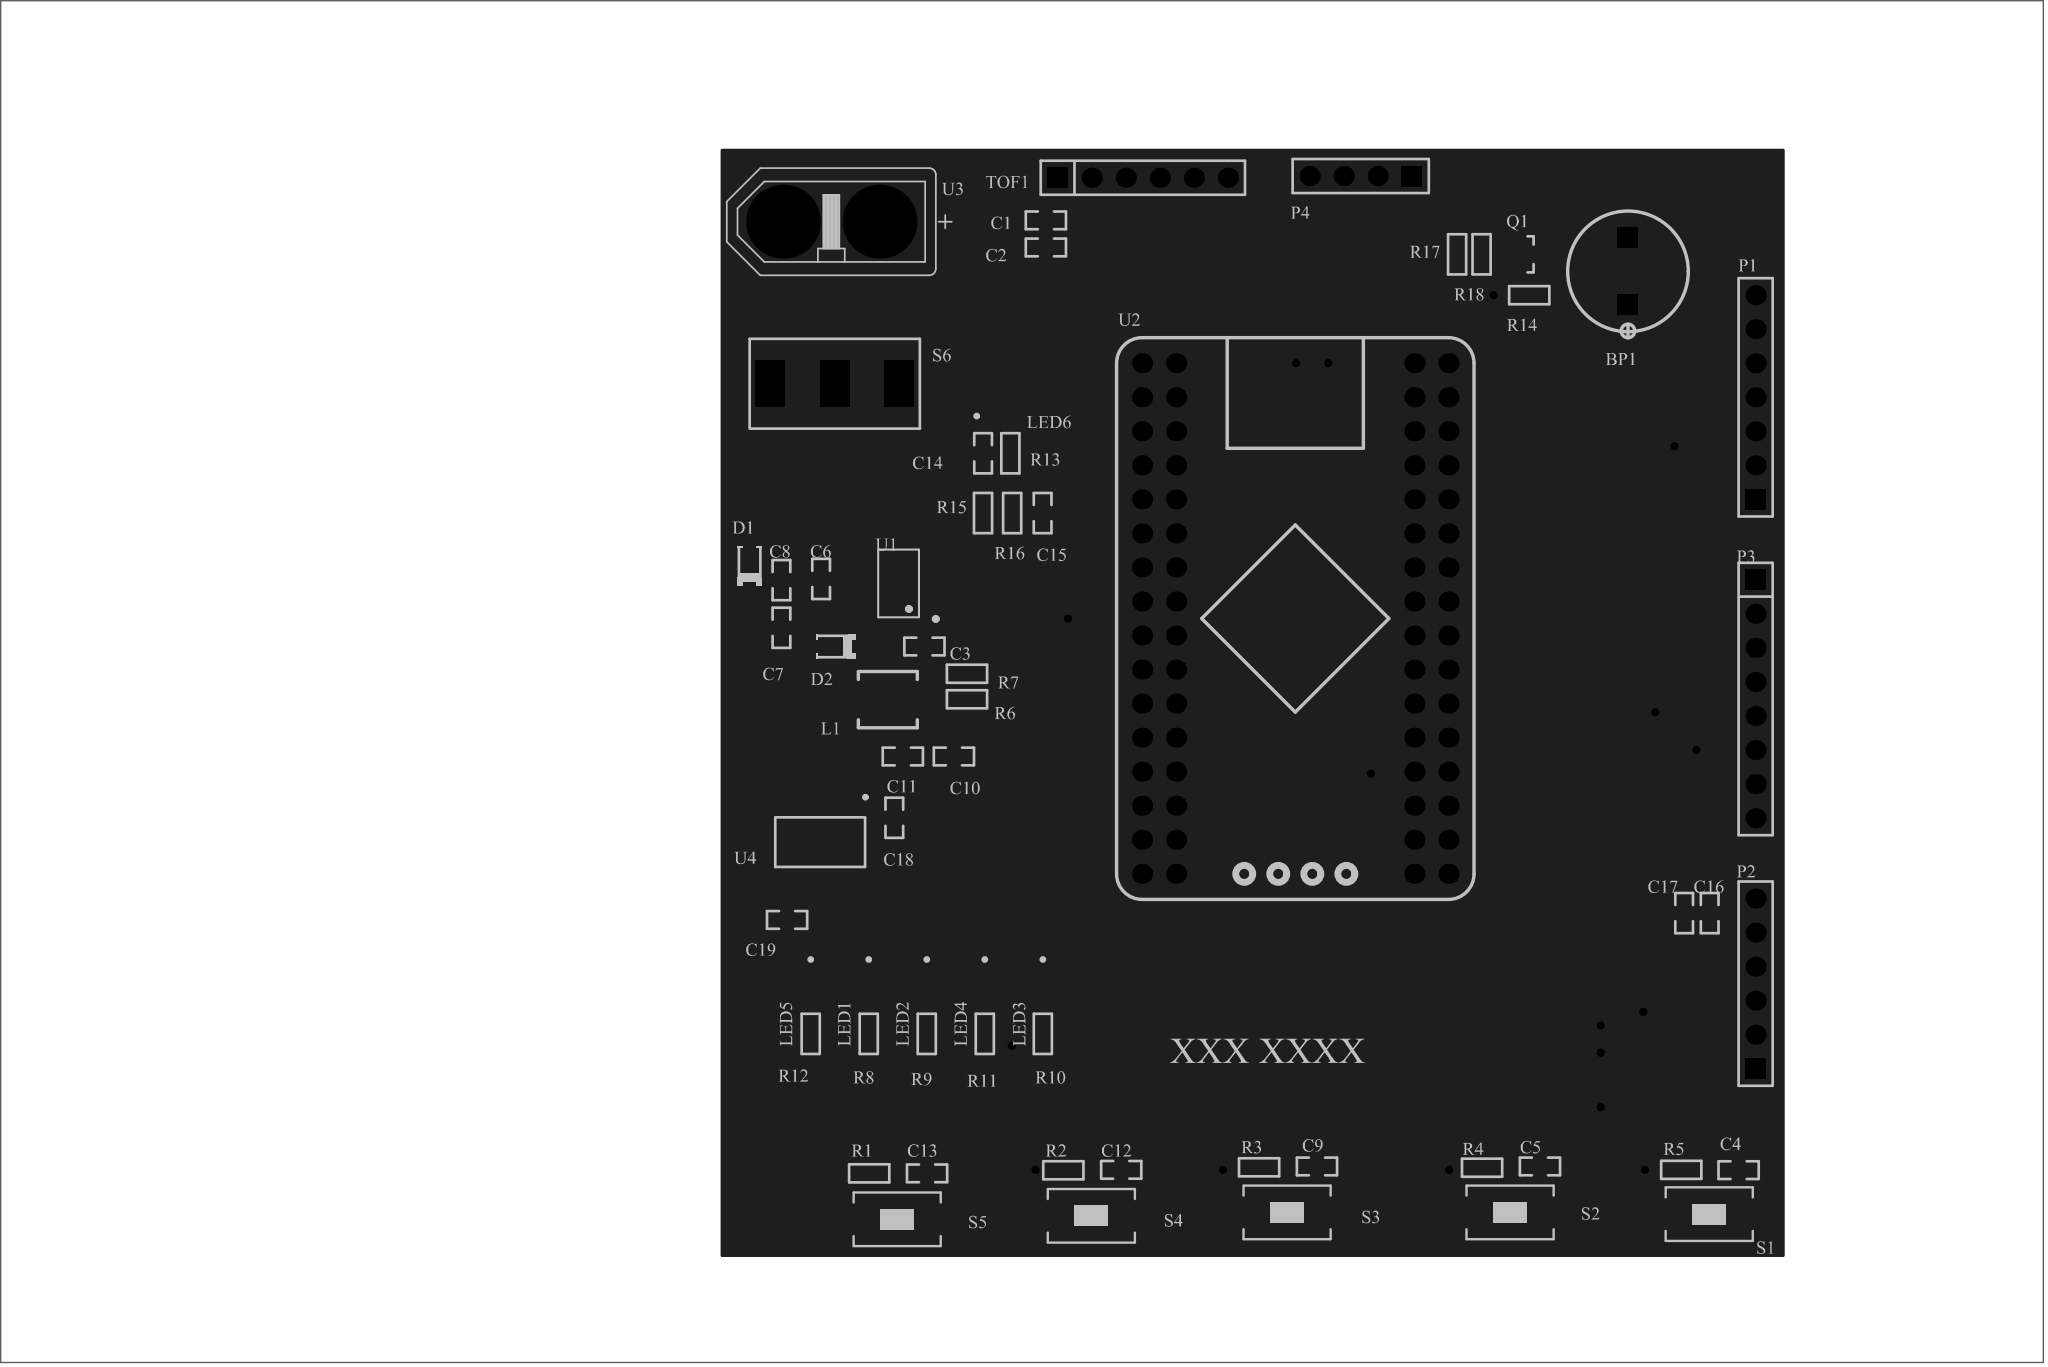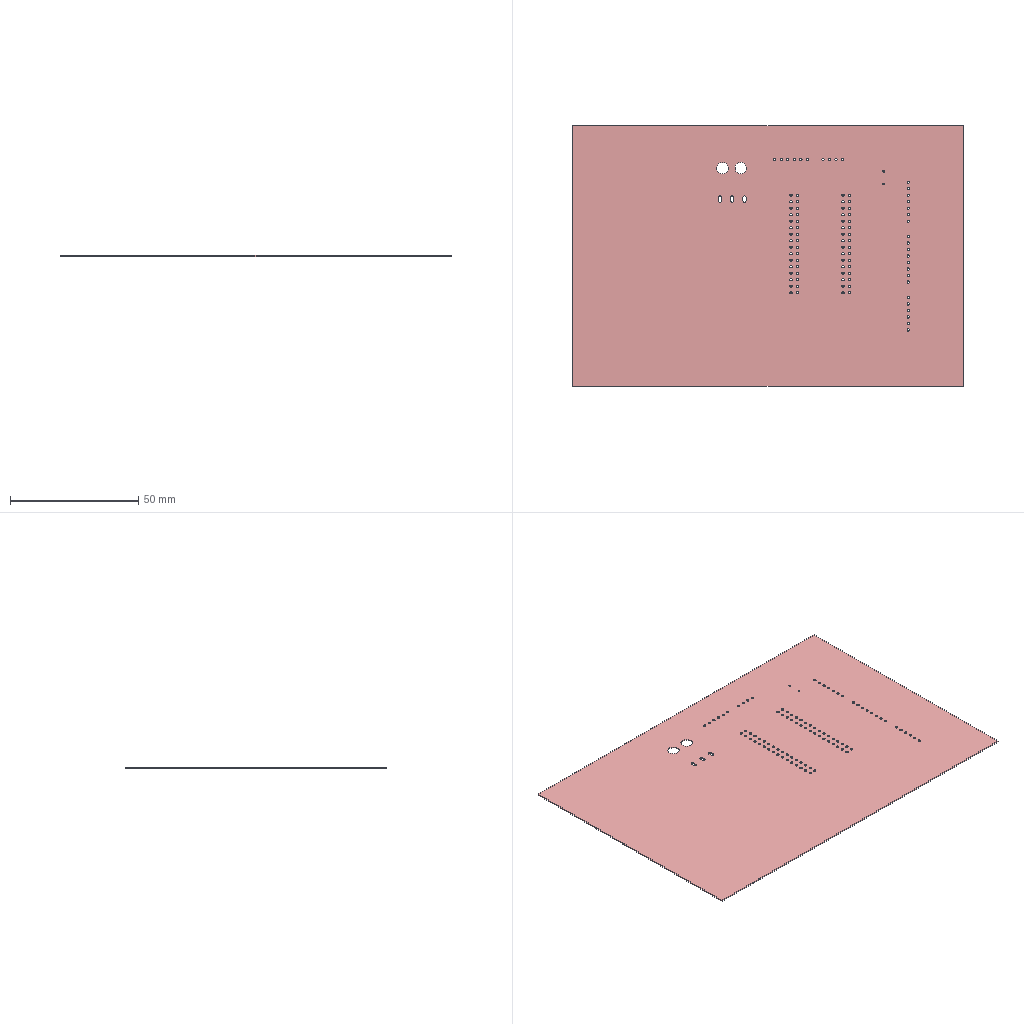Circuit board layout | Altium Designer | box 152.4 x 101.6 x 0.4 mm
Layer stack:
# Altium Designer layer stack of  (unit mm; dielectric type: 0 none, 1 core, 2 prepreg, 3 surface material)
index,name,kind,layer,copper_thickness_mm,dielectric_type,dielectric_thickness_mm,dielectric_material,dielectric_constant
0,Top Paste Mask Layer,other,,,,,,
1,Top Silkscreen Layer,other,,,,,,
2,Top Solder Mask Layer,dielectric,,,3,0.0102,Solder Resist,3.5
3,Top Layer,copper,Top Layer,0.0356,,,,
4,Dielectric 1,dielectric,,,3,0.32,FR-4,4.8
5,Bottom Layer,copper,Bottom Layer,0.0356,,,,
6,Bottom Solder Mask Layer,dielectric,,,3,0.0102,Solder Resist,3.5
7,Bottom Silkscreen Layer,other,,,,,,
8,Bottom Paste Mask Layer,other,,,,,,
# drill layer pairs: low layer,high layer
drill_pair,Top Layer,Bottom Layer
Part placement:
Designator,Comment,Layer,Footprint,Center-X(mm),Center-Y(mm),Rotation
U4,LM1117,TopLayer,LM1117_-_duplicate,137.342,115.023,180
U3,XT60-F,TopLayer,XT60,138.174,161.311,0
U2,STC32G12K128,TopLayer,STC16F40K128_CoreBoard,172.791,131.705,0
U1,TPS5450,TopLayer,5450,143.193,134.324,90
TOF1,Ranging module,TopLayer,HDR1X6,161.417,164.592,0
S6,SW,TopLayer,SS12D10,138.43,149.225,0
S5,KEY,TopLayer,anjiantiepiankaiguan,143.087,86.882,0
S4,KEY,TopLayer,anjiantiepiankaiguan,157.573,87.144,0
S3,KEY,TopLayer,anjiantiepiankaiguan,172.178,87.398,0
S2,KEY,TopLayer,anjiantiepiankaiguan,188.815,87.398,0
S1,KEY,TopLayer,anjiantiepiankaiguan,203.674,87.271,0
R18,10K ±1%,TopLayer,RESC1608[0603]S-N,186.69,158.877,270
R17,4.7K ±1%,TopLayer,RESC1608[0603]S-N,184.863,158.878,90
R16,1K ±1%,TopLayer,RESC1608[0603]S-N,151.667,139.573,90
R15,10K ±1%,TopLayer,RESC1608[0603]S-N,149.494,139.573,270
R14,10R ±1%,TopLayer,RESC1608[0603]S-N,190.246,155.829,0
R13,1K,TopLayer,RESC1608[0603]S-N,151.533,144.036,90
R12,10K,TopLayer,RESC1608[0603]S-N,136.636,100.718,90
R11,10K,TopLayer,RESC1608[0603]S-N,149.626,100.718,90
R10,10K,TopLayer,RESC1608[0603]S-N,153.956,100.718,90
R9,10K,TopLayer,RESC1608[0603]S-N,145.296,100.718,90
R8,10K,TopLayer,RESC1608[0603]S-N,140.966,100.718,90
R7,3K,TopLayer,RESC1608[0603]S-N,148.296,127.586,180
R6,10K,TopLayer,RESC1608[0603]S-N,148.296,125.681,180
R5,1K,TopLayer,RESC1608[0603]S-N,201.586,90.573,180
R4,1K,TopLayer,RESC1608[0603]S-N,186.727,90.731,180
R3,1K,TopLayer,RESC1608[0603]S-N,170.09,90.763,180
R2,1K,TopLayer,RESC1608[0603]S-N,155.485,90.541,180
R1,1K,TopLayer,RESC1608[0603]S-N,140.999,90.311,180
Q1,S8050,TopLayer,SOT-23,189.987,158.878,0
P4,Header-D-M 1x4P,TopLayer,HDR1X4,177.673,164.719,180
P3,Header  1X8,TopLayer,HDR1X8,207.137,125.702,270
P2,Gyroscope,TopLayer,HDR1X6,207.137,104.465,90
P1,Header 7,TopLayer,HDR1X7,207.137,148.209,90
LED6,LED,TopLayer,LEDC1608(0603),150.622,146.812,0
LED5,LED,TopLayer,LEDC1608(0603),136.636,104.667,270
LED4,LED,TopLayer,LEDC1608(0603),149.626,104.667,270
LED3,LED,TopLayer,LEDC1608(0603),153.956,104.667,270
LED2,LED,TopLayer,LEDC1608(0603),145.296,104.667,270
LED1,LED,TopLayer,LEDC1608(0603),140.966,104.667,270
L1,4.7uH 2.5A,TopLayer,0402_TPC_4*4*2,142.389,125.655,270
D2,SS54,TopLayer,SOD-123-L,138.517,129.618,0
D1,SS54,TopLayer,SOD-123-L,132.08,135.636,270
C19,1uF,TopLayer,CAPC1608[0603]S-N,134.874,109.22,0
C18,1uF,TopLayer,CAPC1608[0603]S-N,142.875,116.84,270
C17,10uF ±10% 50V,TopLayer,CAPC1608[0603]S-N,201.803,109.728,270
C16,0.1uF ±10% 25V,TopLayer,CAPC1608[0603]S-N,203.708,109.728,270
C15,100nF 50V X7R,TopLayer,CAPC1608[0603]S-N,153.939,139.573,90
C14,1000uF  25V,TopLayer,CAPC1608[0603]S-N,149.498,144.036,90
C13,10uF,TopLayer,CAPC1608[0603]S-N,145.317,90.311,0
C12,10uF,TopLayer,CAPC1608[0603]S-N,159.803,90.573,0
C11,0.1uF,TopLayer,CAPC1608[0603]S-N,143.51,121.412,0
C10,100uF,TopLayer,CAPC1608[0603]S-N,147.32,121.412,0
C9,10uF,TopLayer,CAPC1608[0603]S-N,174.408,90.827,0
C8,4.7uF,TopLayer,CAPC1608[0603]S-N,134.453,134.571,270
C7,4.7uF,TopLayer,CAPC1608[0603]S-N,134.453,131.015,90
C6,0.1uF,TopLayer,CAPC1608[0603]S-N,137.413,134.659,270
C5,10uF,TopLayer,CAPC1608[0603]S-N,191.045,90.827,0
C4,10uF,TopLayer,CAPC1608[0603]S-N,205.867,90.551,0
C3,100nF,TopLayer,CAPC1608[0603]S-N,145.121,129.618,180
C2,0.1uF,TopLayer,CAPC1608[0603]S-N,154.182,159.391,0
C1,10uF,TopLayer,CAPC1608[0603]S-N,154.182,161.412,0
BP1,Buzzer,TopLayer,5*10fengmiqi,197.612,157.607,90
Pad and via stacks:
# Altium Designer via and pad stacks of  (unit mm). Each distinct definition once, with the count of objects using it.
# via: kind,start_layer,end_layer,hole_mm,diameter_mm,mode(0 simple;1 top-mid-bottom;2 full stack),diameter_per_layer,count,example_net
# pad: kind,layer,hole_mm,hole_type(0 round;1 square;2 slot),plating,top_size,top_shape(1 round;2 rect;3 octagon;9 rounded rect),mid_size,bottom_size,mode,footprint,size_per_layer,count,example
pad,Top Layer,0,0,plated,1.1x1.55,2,1.1x1.55,1.1x1.55,0,LM1117 - duplicate,,3,U4.2
pad,Top Layer,0,0,plated,3.45x1.55,2,3.45x1.55,3.45x1.55,0,LM1117 - duplicate,,1,U4.4
pad,Top Layer,0,0,plated,0.6x1.8,1,0.6x1.8,0.6x1.8,0,5450,,8,U1.1
pad,Top Layer,0,0,plated,2.29x2.29,2,2.29x2.29,2.29x2.29,0,5450,,1,U1.9
pad,Top Layer,0,0,plated,2.5x2,2,2.5x2,2.5x2,0,anjiantiepiankaiguan,,10,S5.2
pad,Top Layer,0,0,plated,0.95x0.9,2,0.95x0.9,0.95x0.9,0,RESC1608[0603]S-N,,36,R18.2
pad,Top Layer,0,0,plated,0.65x1.05,2,0.65x1.05,0.65x1.05,0,SOT-23,,3,Q1.3
pad,Top Layer,0,0,unplated,0.8x0.85,2,0.8x0.85,0.8x0.85,0,LEDC1608(0603),,12,LED6.A
pad,Top Layer,0,2,plated,1.5x2.5,2,1.5x2.5,1.5x2.5,0,0402 TPC 4*4*2,,2,L1.2
pad,Top Layer,0,0,unplated,1x0.85,2,1x0.85,1x0.85,0,SOD-123-L,,4,D2.K
pad,Top Layer,0,0,plated,0.95x0.9,2,0.95x0.9,0.95x0.9,0,CAPC1608[0603]S-N,,38,C19.1
pad,Multi-Layer,4.5,2,plated,5.516x5.516,1,5.516x5.516,5.516x5.516,0,XT60,,2,U3.
pad,Multi-Layer,0.9,0,plated,1.5x1.5,1,1.5x1.5,1.5x1.5,0,STC16F40K128_CoreBoard,,64,U2.40
pad,Multi-Layer,0.9,0,plated,1.5x1.5,1,1.5x1.5,1.5x1.5,0,HDR1X6,,10,TOF1.6
pad,Multi-Layer,0.9,0,plated,1.5x1.5,2,1.5x1.5,1.5x1.5,0,HDR1X6,,2,TOF1.1
pad,Multi-Layer,1.2,2,plated,2.2x3.5,2,2.2x3.5,2.2x3.5,0,SS12D10,,3,S6.3
pad,Multi-Layer,0.9,0,plated,1.5x1.5,1,1.5x1.5,1.5x1.5,0,HDR1X4,,3,P4.4
pad,Multi-Layer,0.9,0,plated,1.5x1.5,2,1.5x1.5,1.5x1.5,0,HDR1X4,,1,P4.1
pad,Multi-Layer,0.9,0,plated,1.5x1.5,1,1.5x1.5,1.5x1.5,0,HDR1X8,,7,P3.8
pad,Multi-Layer,0.9,0,plated,1.5x1.5,2,1.5x1.5,1.5x1.5,0,HDR1X8,,1,P3.1
pad,Multi-Layer,0.9,0,plated,1.5x1.5,1,1.5x1.5,1.5x1.5,0,HDR1X7,,6,P1.7
pad,Multi-Layer,0.9,0,plated,1.5x1.5,2,1.5x1.5,1.5x1.5,0,HDR1X7,,1,P1.1
pad,Multi-Layer,0.762,0,plated,1.524x1.524,2,1.524x1.524,1.524x1.524,0,5*10fengmiqi,,2,BP1.2
via,Top Layer,Bottom Layer,0.3048,0.61,0,,17,23
Copper pours:
name,layer,net,type(0 solid;1 hatched;2 none)
Top Layer-GND,Top Layer,GND,0
Bottom Layer-GND,Bottom Layer,GND,0
Design rules, without the lines most boards share:
# Altium Designer design rules of  (exported by Altium Designer, unit mm)
# columns: name | kind | enabled | priority | scope1 | scope2 | descriptor | typed fields (field=value)
ComponentClearance_1 | 24 | enabled | 1 | All | All | Component Clearance Constraint ( Horizontal Gap = 10mil, Vertical Gap = 10mil ) (All),(All)  | gap=0.254
Clearance | 0 | enabled | 1 | All | All | Clearance Constraint (Gap=5mil) (All),(All) | gap=0.127
Clearance_1 | 63 | enabled | 1 | All | All | Board Clearance Constraint (Gap=0mil) (All) |
ComponentClearance | 52 | enabled | 1 | All | All | Hole To Hole Clearance (Gap=10mil) (All),(All) | gap=0.254
Width | 2 | enabled | 1 | All | All | Width Constraint (Min=10mil) (Max=200mil) (Preferred=10mil) (All) |
DiffPairsRouting | 51 | enabled | 1 | All | All | Differential Pairs Uncoupled Length using the Gap Constraints (Min=10mil) (Max=10mil) (Prefered=10mil)  and Width Constraints (Min=15mil) (Max=15mil) (Prefered=15mil) (All) |
RoutingVias | 11 | enabled | 1 | All | All | Routing Via (MinHoleWidth=2mil) (MaxHoleWidth=28mil) (PreferredHoleWidth=28mil) (MinWidth=2mil) (MaxWidth=50mil) (PreferedWidth=50mil) (All) | via_min_hole=0.0508 via_max_hole=0.7112 via_preferred_diameter=1.27 via_preferred_hole=0.7112
PlaneConnect | 6 | enabled | 1 | All | All | Power Plane Connect Rule(Direct Connect )(Expansion=20mil) (Conductor Width=10mil) (Air Gap=10mil) (Entries=4) (All) | relief_conductor_width=0.254 relief_entries=4 relief_expansion=0.508
PolygonConnect | 20 | enabled | 1 | (InNet('GND')) | All | Polygon Connect Rule(Direct Connect )(Conductor Width=10mil) (Relief Angle=90 Angle) (Entries=4) (Air Gap Width=10mil) ((InNet('GND'))),(All) | connect_style(0=relief,1=direct,2=none)=1 relief_conductor_width=0.254 relief_entries=4
PasteMaskExpansion | 14 | enabled | 1 | All | All | Paste Mask Expansion (Expansion =0mil) (All) | expansion=0
SolderMaskExpansion | 13 | enabled | 1 | All | All | Solder Mask Expansion (Expansion =4mil) (All) | expansion=0.1016